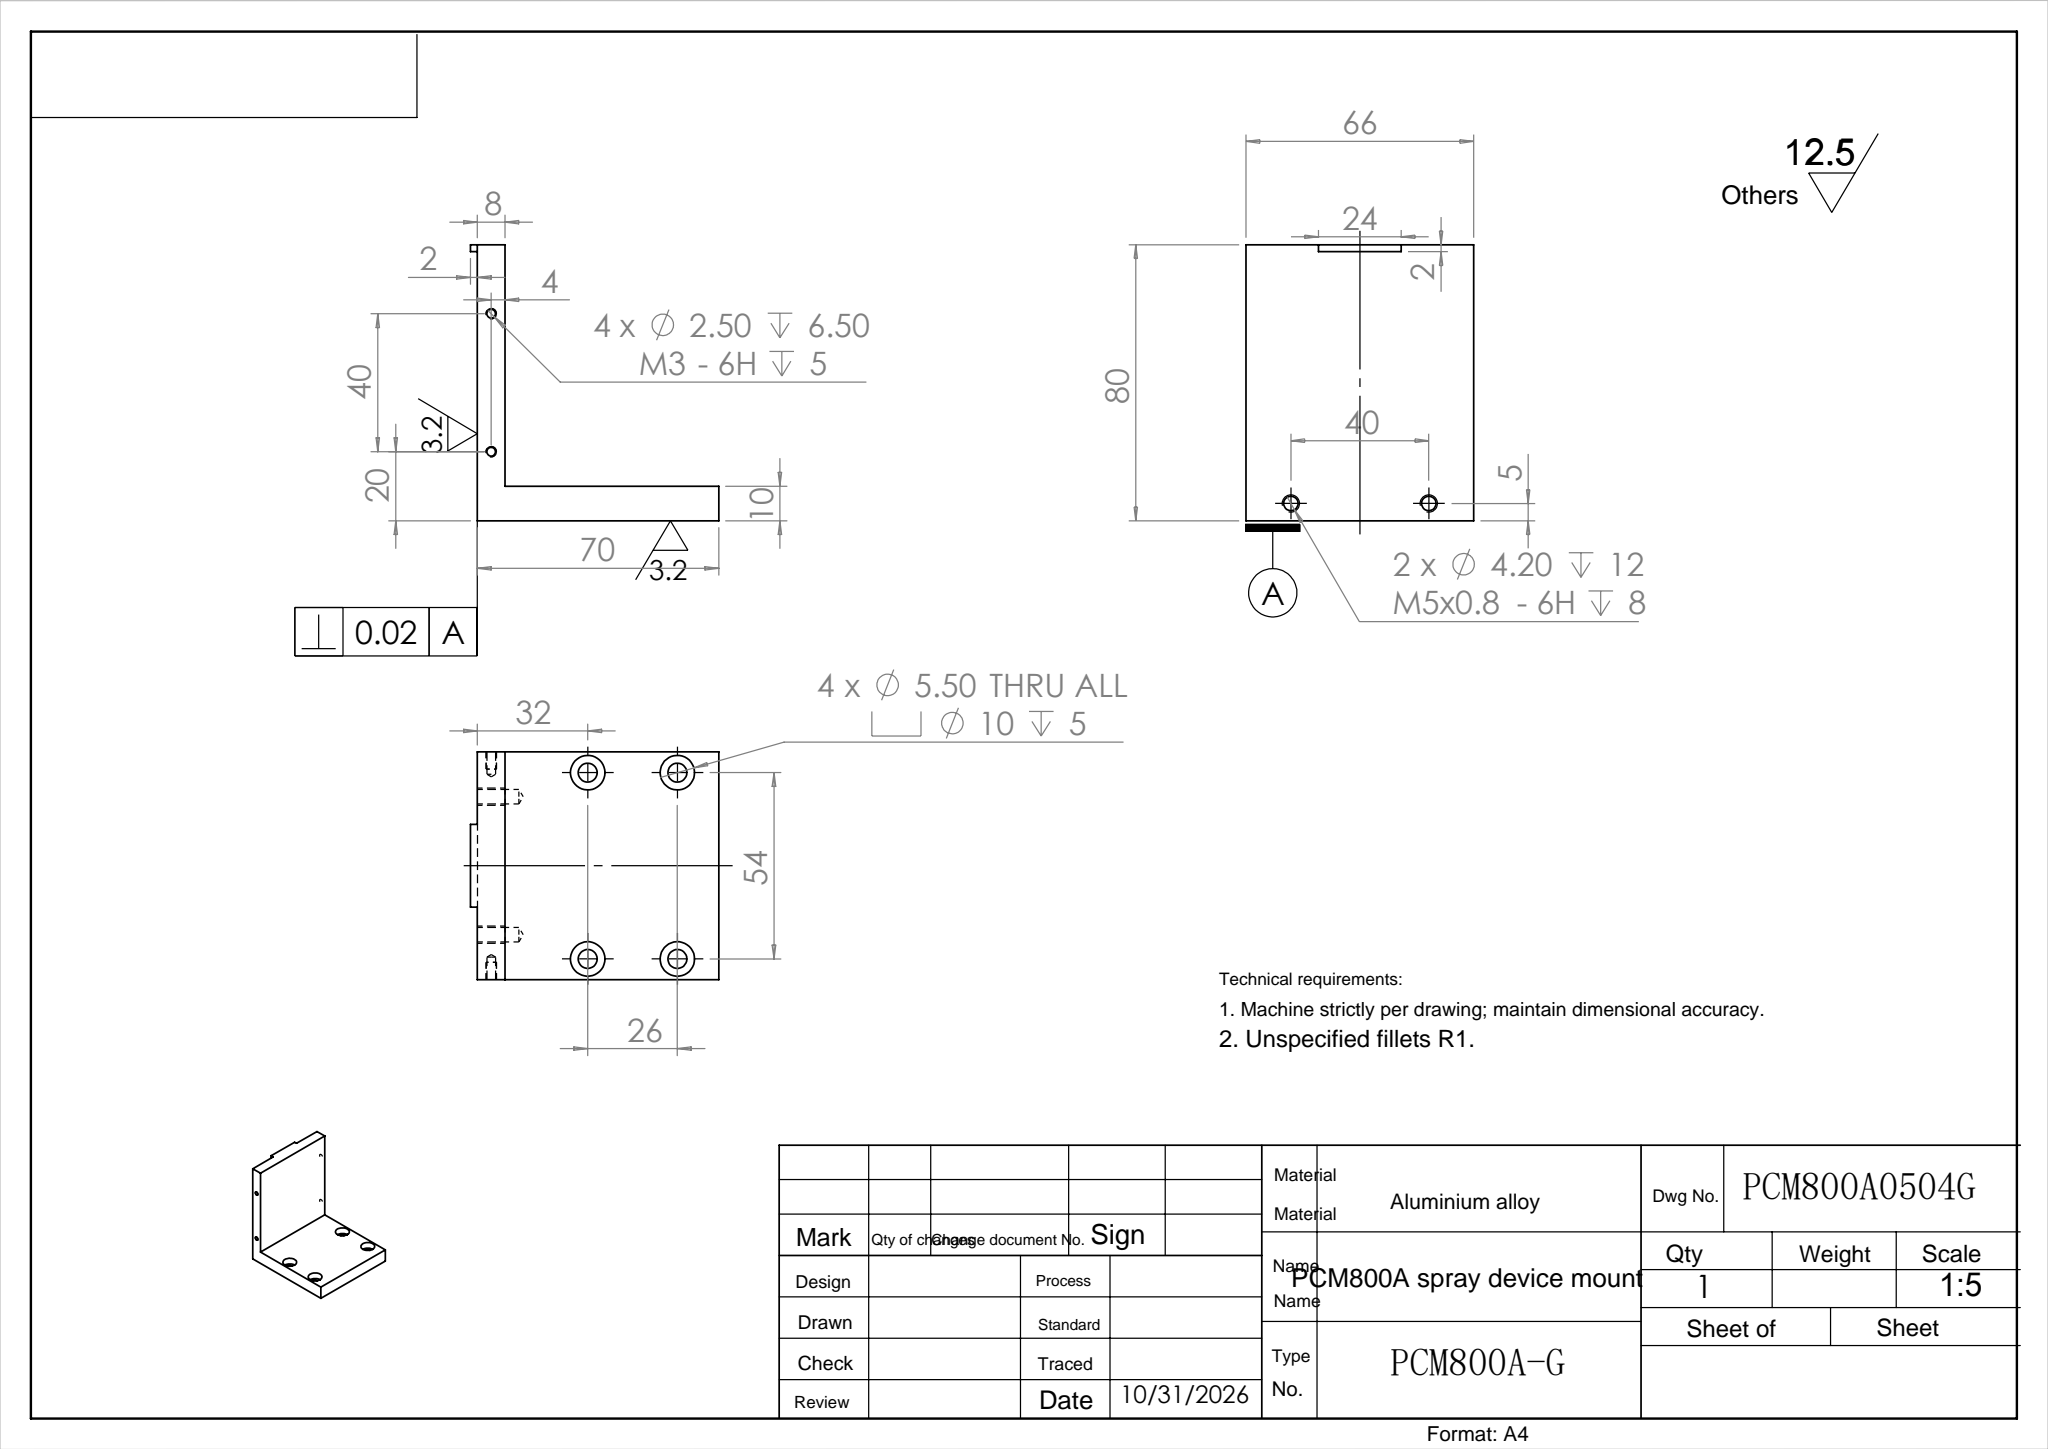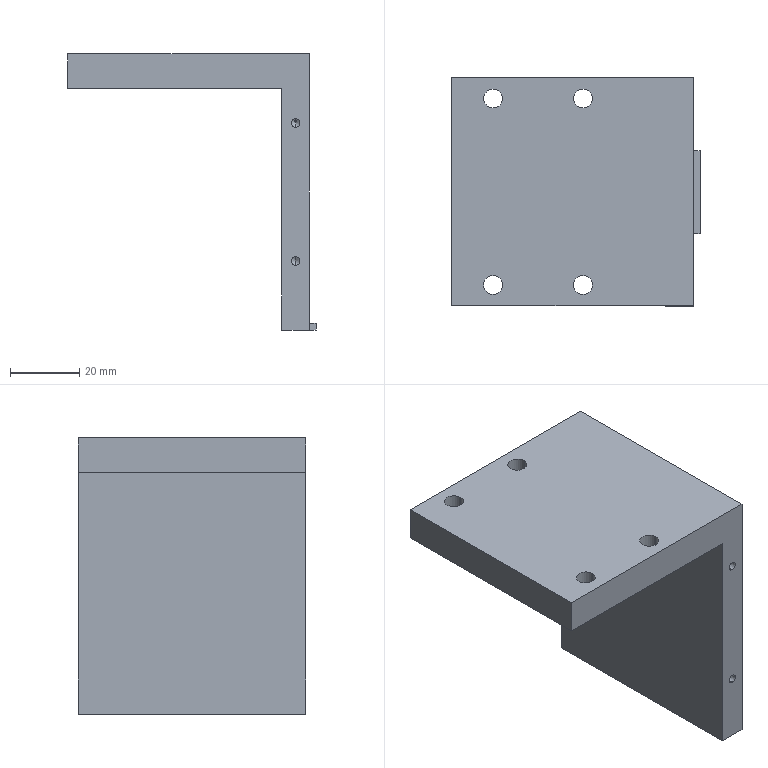Part | SolidWorks | features Boss 3, HoleWzd 3, Extrusion 1, MirrorPattern 1 | 1 solid | 56 faces | box 72 x 66 x 80 mm | volume 80733 mm3 | cylinder 28 | plane 16 | cone 12 | commonest cylinder face diameters 2.5 x8 5.5 x8 10 x8 4.2 x4